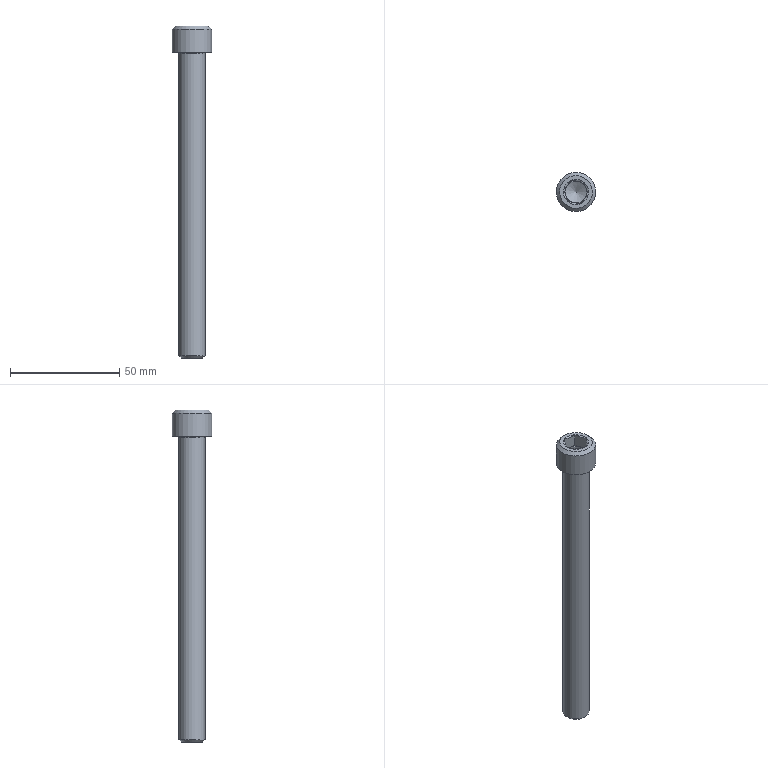Part | NX | features solid 2 | 1 solid | 32 faces | box 18 x 18 x 152 mm | volume 18123 mm3 | plane 19 | cone 9 | cylinder 3 | torus 1 | commonest cylinder face diameters 10 x1 12 x1 18 x1
STEP:
#1=CARTESIAN_POINT('',(532.671,620.304,196.));
#2=VERTEX_POINT('',#1);
#3=CARTESIAN_POINT('',(531.842,622.582,196.));
#4=VERTEX_POINT('',#3);
#5=CARTESIAN_POINT('',(533.817,617.157,196.));
#6=DIRECTION('',(-0.342,0.9397,0.));
#7=VECTOR('',#6,1000.);
#8=LINE('',#5,#7);
#9=EDGE_CURVE('',#2,#4,#8,.T.);
#10=ORIENTED_EDGE('',*,*,#9,.T.);
#11=CARTESIAN_POINT('',(529.455,623.003,196.));
#12=VERTEX_POINT('',#11);
#13=CARTESIAN_POINT('',(526.156,623.585,196.));
#14=DIRECTION('',(0.9848,-0.1736,0.));
#15=VECTOR('',#14,1000.);
#16=LINE('',#13,#15);
#17=EDGE_CURVE('',#12,#4,#16,.T.);
#18=ORIENTED_EDGE('',*,*,#17,.F.);
#19=CARTESIAN_POINT('',(528.146,618.178,196.));
#20=DIRECTION('',(0.,0.,1.));
#21=DIRECTION('',(0.766,-0.6428,0.));
#22=AXIS2_PLACEMENT_3D('',#19,#20,#21);
#23=CIRCLE('',#22,5.);
#24=EDGE_CURVE('',#2,#12,#23,.T.);
#25=ORIENTED_EDGE('',*,*,#24,.F.);
#26=EDGE_LOOP('',(#10,#18,#25));
#27=FACE_BOUND('',#26,.T.);
#28=CARTESIAN_POINT('',(528.146,618.178,196.));
#29=DIRECTION('',(0.,0.,1.));
#30=DIRECTION('',(-0.766,0.6428,0.));
#31=AXIS2_PLACEMENT_3D('',#28,#29,#30);
#32=PLANE('',#31);
#33=ADVANCED_FACE('',(#27),#32,.T.);
#34=CARTESIAN_POINT('',(526.156,623.585,196.));
#35=VERTEX_POINT('',#34);
#36=CARTESIAN_POINT('',(528.567,623.16,196.));
#37=VERTEX_POINT('',#36);
#38=CARTESIAN_POINT('',(526.156,623.585,196.));
#39=DIRECTION('',(0.9848,-0.1736,0.));
#40=VECTOR('',#39,1000.);
#41=LINE('',#38,#40);
#42=EDGE_CURVE('',#35,#37,#41,.T.);
#43=ORIENTED_EDGE('',*,*,#42,.F.);
#44=CARTESIAN_POINT('',(524.316,621.391,196.));
#45=VERTEX_POINT('',#44);
#46=CARTESIAN_POINT('',(522.475,619.198,196.));
#47=DIRECTION('',(0.6428,0.766,0.));
#48=VECTOR('',#47,1000.);
#49=LINE('',#46,#48);
#50=EDGE_CURVE('',#45,#35,#49,.T.);
#51=ORIENTED_EDGE('',*,*,#50,.F.);
#52=CARTESIAN_POINT('',(528.146,618.178,196.));
#53=DIRECTION('',(0.,0.,1.));
#54=DIRECTION('',(0.766,-0.6428,0.));
#55=AXIS2_PLACEMENT_3D('',#52,#53,#54);
#56=CIRCLE('',#55,5.);
#57=EDGE_CURVE('',#37,#45,#56,.T.);
#58=ORIENTED_EDGE('',*,*,#57,.F.);
#59=EDGE_LOOP('',(#43,#51,#58));
#60=FACE_BOUND('',#59,.T.);
#61=CARTESIAN_POINT('',(528.146,618.178,196.));
#62=DIRECTION('',(0.,0.,1.));
#63=DIRECTION('',(-0.766,0.6428,0.));
#64=AXIS2_PLACEMENT_3D('',#61,#62,#63);
#65=PLANE('',#64);
#66=ADVANCED_FACE('',(#60),#65,.T.);
#67=CARTESIAN_POINT('',(522.475,619.198,196.));
#68=VERTEX_POINT('',#67);
#69=CARTESIAN_POINT('',(522.475,619.198,196.));
#70=DIRECTION('',(0.6428,0.766,0.));
#71=VECTOR('',#70,1000.);
#72=LINE('',#69,#71);
#73=EDGE_CURVE('',#68,#45,#72,.T.);
#74=ORIENTED_EDGE('',*,*,#73,.F.);
#75=CARTESIAN_POINT('',(523.312,616.898,196.));
#76=VERTEX_POINT('',#75);
#77=CARTESIAN_POINT('',(524.45,613.773,196.));
#78=DIRECTION('',(-0.342,0.9397,0.));
#79=VECTOR('',#78,1000.);
#80=LINE('',#77,#79);
#81=EDGE_CURVE('',#76,#68,#80,.T.);
#82=ORIENTED_EDGE('',*,*,#81,.F.);
#83=CARTESIAN_POINT('',(528.146,618.178,196.));
#84=DIRECTION('',(0.,0.,1.));
#85=DIRECTION('',(0.766,-0.6428,0.));
#86=AXIS2_PLACEMENT_3D('',#83,#84,#85);
#87=CIRCLE('',#86,5.);
#88=EDGE_CURVE('',#45,#76,#87,.T.);
#89=ORIENTED_EDGE('',*,*,#88,.F.);
#90=EDGE_LOOP('',(#74,#82,#89));
#91=FACE_BOUND('',#90,.T.);
#92=CARTESIAN_POINT('',(528.146,618.178,196.));
#93=DIRECTION('',(0.,0.,1.));
#94=DIRECTION('',(-0.766,0.6428,0.));
#95=AXIS2_PLACEMENT_3D('',#92,#93,#94);
#96=PLANE('',#95);
#97=ADVANCED_FACE('',(#91),#96,.T.);
#98=CARTESIAN_POINT('',(524.45,613.773,196.));
#99=VERTEX_POINT('',#98);
#100=CARTESIAN_POINT('',(523.621,616.051,196.));
#101=VERTEX_POINT('',#100);
#102=CARTESIAN_POINT('',(524.45,613.773,196.));
#103=DIRECTION('',(-0.342,0.9397,0.));
#104=VECTOR('',#103,1000.);
#105=LINE('',#102,#104);
#106=EDGE_CURVE('',#99,#101,#105,.T.);
#107=ORIENTED_EDGE('',*,*,#106,.F.);
#108=CARTESIAN_POINT('',(526.837,613.352,196.));
#109=VERTEX_POINT('',#108);
#110=CARTESIAN_POINT('',(530.136,612.77,196.));
#111=DIRECTION('',(-0.9848,0.1736,0.));
#112=VECTOR('',#111,1000.);
#113=LINE('',#110,#112);
#114=EDGE_CURVE('',#109,#99,#113,.T.);
#115=ORIENTED_EDGE('',*,*,#114,.F.);
#116=CARTESIAN_POINT('',(528.146,618.178,196.));
#117=DIRECTION('',(0.,0.,1.));
#118=DIRECTION('',(0.766,-0.6428,0.));
#119=AXIS2_PLACEMENT_3D('',#116,#117,#118);
#120=CIRCLE('',#119,5.);
#121=EDGE_CURVE('',#101,#109,#120,.T.);
#122=ORIENTED_EDGE('',*,*,#121,.F.);
#123=EDGE_LOOP('',(#107,#115,#122));
#124=FACE_BOUND('',#123,.T.);
#125=CARTESIAN_POINT('',(528.146,618.178,196.));
#126=DIRECTION('',(0.,0.,1.));
#127=DIRECTION('',(-0.766,0.6428,0.));
#128=AXIS2_PLACEMENT_3D('',#125,#126,#127);
#129=PLANE('',#128);
#130=ADVANCED_FACE('',(#124),#129,.T.);
#131=CARTESIAN_POINT('',(533.817,617.157,196.));
#132=VERTEX_POINT('',#131);
#133=CARTESIAN_POINT('',(531.976,614.964,196.));
#134=VERTEX_POINT('',#133);
#135=CARTESIAN_POINT('',(533.817,617.157,196.));
#136=DIRECTION('',(-0.6428,-0.766,0.));
#137=VECTOR('',#136,1000.);
#138=LINE('',#135,#137);
#139=EDGE_CURVE('',#132,#134,#138,.T.);
#140=ORIENTED_EDGE('',*,*,#139,.F.);
#141=CARTESIAN_POINT('',(532.979,619.457,196.));
#142=VERTEX_POINT('',#141);
#143=CARTESIAN_POINT('',(533.817,617.157,196.));
#144=DIRECTION('',(-0.342,0.9397,0.));
#145=VECTOR('',#144,1000.);
#146=LINE('',#143,#145);
#147=EDGE_CURVE('',#132,#142,#146,.T.);
#148=ORIENTED_EDGE('',*,*,#147,.T.);
#149=CARTESIAN_POINT('',(528.146,618.178,196.));
#150=DIRECTION('',(0.,0.,1.));
#151=DIRECTION('',(0.766,-0.6428,0.));
#152=AXIS2_PLACEMENT_3D('',#149,#150,#151);
#153=CIRCLE('',#152,5.);
#154=EDGE_CURVE('',#134,#142,#153,.T.);
#155=ORIENTED_EDGE('',*,*,#154,.F.);
#156=EDGE_LOOP('',(#140,#148,#155));
#157=FACE_BOUND('',#156,.T.);
#158=CARTESIAN_POINT('',(528.146,618.178,196.));
#159=DIRECTION('',(0.,0.,1.));
#160=DIRECTION('',(-0.766,0.6428,0.));
#161=AXIS2_PLACEMENT_3D('',#158,#159,#160);
#162=PLANE('',#161);
#163=ADVANCED_FACE('',(#157),#162,.T.);
#164=CARTESIAN_POINT('',(530.136,612.77,196.));
#165=VERTEX_POINT('',#164);
#166=CARTESIAN_POINT('',(527.725,613.195,196.));
#167=VERTEX_POINT('',#166);
#168=CARTESIAN_POINT('',(530.136,612.77,196.));
#169=DIRECTION('',(-0.9848,0.1736,0.));
#170=VECTOR('',#169,1000.);
#171=LINE('',#168,#170);
#172=EDGE_CURVE('',#165,#167,#171,.T.);
#173=ORIENTED_EDGE('',*,*,#172,.F.);
#174=CARTESIAN_POINT('',(533.817,617.157,196.));
#175=DIRECTION('',(-0.6428,-0.766,0.));
#176=VECTOR('',#175,1000.);
#177=LINE('',#174,#176);
#178=EDGE_CURVE('',#134,#165,#177,.T.);
#179=ORIENTED_EDGE('',*,*,#178,.F.);
#180=CARTESIAN_POINT('',(528.146,618.178,196.));
#181=DIRECTION('',(0.,0.,1.));
#182=DIRECTION('',(0.766,-0.6428,0.));
#183=AXIS2_PLACEMENT_3D('',#180,#181,#182);
#184=CIRCLE('',#183,5.);
#185=EDGE_CURVE('',#167,#134,#184,.T.);
#186=ORIENTED_EDGE('',*,*,#185,.F.);
#187=EDGE_LOOP('',(#173,#179,#186));
#188=FACE_BOUND('',#187,.T.);
#189=CARTESIAN_POINT('',(528.146,618.178,196.));
#190=DIRECTION('',(0.,0.,1.));
#191=DIRECTION('',(-0.766,0.6428,0.));
#192=AXIS2_PLACEMENT_3D('',#189,#190,#191);
#193=PLANE('',#192);
#194=ADVANCED_FACE('',(#188),#193,.T.);
#195=CARTESIAN_POINT('',(522.475,619.198,202.));
#196=VERTEX_POINT('',#195);
#197=CARTESIAN_POINT('',(522.491,619.216,202.));
#198=VERTEX_POINT('',#197);
#199=CARTESIAN_POINT('',(522.475,619.198,202.));
#200=DIRECTION('',(0.6428,0.766,0.));
#201=VECTOR('',#200,1000.);
#202=LINE('',#199,#201);
#203=EDGE_CURVE('',#196,#198,#202,.T.);
#204=ORIENTED_EDGE('',*,*,#203,.F.);
#205=CARTESIAN_POINT('',(522.475,619.198,196.));
#206=DIRECTION('',(0.,0.,1.));
#207=VECTOR('',#206,1000.);
#208=LINE('',#205,#207);
#209=EDGE_CURVE('',#68,#196,#208,.T.);
#210=ORIENTED_EDGE('',*,*,#209,.F.);
#211=ORIENTED_EDGE('',*,*,#73,.T.);
#212=ORIENTED_EDGE('',*,*,#50,.T.);
#213=CARTESIAN_POINT('',(526.156,623.585,202.));
#214=VERTEX_POINT('',#213);
#215=CARTESIAN_POINT('',(526.156,623.585,196.));
#216=DIRECTION('',(0.,0.,1.));
#217=VECTOR('',#216,1000.);
#218=LINE('',#215,#217);
#219=EDGE_CURVE('',#35,#214,#218,.T.);
#220=ORIENTED_EDGE('',*,*,#219,.T.);
#221=CARTESIAN_POINT('',(526.141,623.567,202.));
#222=VERTEX_POINT('',#221);
#223=CARTESIAN_POINT('',(522.475,619.198,202.));
#224=DIRECTION('',(0.6428,0.766,0.));
#225=VECTOR('',#224,1000.);
#226=LINE('',#223,#225);
#227=EDGE_CURVE('',#222,#214,#226,.T.);
#228=ORIENTED_EDGE('',*,*,#227,.F.);
#229=CARTESIAN_POINT('',(522.491,619.216,202.));
#230=CARTESIAN_POINT('',(523.084,619.924,201.737));
#231=CARTESIAN_POINT('',(524.315,621.39,201.397));
#232=CARTESIAN_POINT('',(525.551,622.863,201.738));
#233=CARTESIAN_POINT('',(526.141,623.567,202.));
#234=B_SPLINE_CURVE_WITH_KNOTS('',3,(#229,#230,#231,#232,#233),.UNSPECIFIED.,.F.,.F.,(4,1,4),(0.004945,0.007815,0.01069),.UNSPECIFIED.);
#235=EDGE_CURVE('',#198,#222,#234,.T.);
#236=ORIENTED_EDGE('',*,*,#235,.F.);
#237=EDGE_LOOP('',(#204,#210,#211,#212,#220,#228,#236));
#238=FACE_BOUND('',#237,.T.);
#239=CARTESIAN_POINT('',(522.475,619.198,196.));
#240=DIRECTION('',(-0.766,0.6428,0.));
#241=DIRECTION('',(0.,0.,-1.));
#242=AXIS2_PLACEMENT_3D('',#239,#240,#241);
#243=PLANE('',#242);
#244=ADVANCED_FACE('',(#238),#243,.F.);
#245=CARTESIAN_POINT('',(524.45,613.773,202.));
#246=VERTEX_POINT('',#245);
#247=CARTESIAN_POINT('',(524.45,613.773,196.));
#248=DIRECTION('',(0.,0.,1.));
#249=VECTOR('',#248,1000.);
#250=LINE('',#247,#249);
#251=EDGE_CURVE('',#99,#246,#250,.T.);
#252=ORIENTED_EDGE('',*,*,#251,.F.);
#253=ORIENTED_EDGE('',*,*,#106,.T.);
#254=CARTESIAN_POINT('',(524.45,613.773,196.));
#255=DIRECTION('',(-0.342,0.9397,0.));
#256=VECTOR('',#255,1000.);
#257=LINE('',#254,#256);
#258=EDGE_CURVE('',#101,#76,#257,.T.);
#259=ORIENTED_EDGE('',*,*,#258,.T.);
#260=ORIENTED_EDGE('',*,*,#81,.T.);
#261=ORIENTED_EDGE('',*,*,#209,.T.);
#262=CARTESIAN_POINT('',(522.483,619.176,202.));
#263=VERTEX_POINT('',#262);
#264=CARTESIAN_POINT('',(524.45,613.773,202.));
#265=DIRECTION('',(-0.342,0.9397,0.));
#266=VECTOR('',#265,1000.);
#267=LINE('',#264,#266);
#268=EDGE_CURVE('',#263,#196,#267,.T.);
#269=ORIENTED_EDGE('',*,*,#268,.F.);
#270=CARTESIAN_POINT('',(524.45,613.773,202.));
#271=CARTESIAN_POINT('',(524.129,614.655,201.729));
#272=CARTESIAN_POINT('',(523.47,616.465,201.382));
#273=CARTESIAN_POINT('',(522.805,618.293,201.729));
#274=CARTESIAN_POINT('',(522.483,619.176,202.));
#275=B_SPLINE_CURVE_WITH_KNOTS('',3,(#270,#271,#272,#273,#274),.UNSPECIFIED.,.F.,.F.,(4,1,4),(0.000000238,0.002904,0.005807),.UNSPECIFIED.);
#276=EDGE_CURVE('',#246,#263,#275,.T.);
#277=ORIENTED_EDGE('',*,*,#276,.F.);
#278=EDGE_LOOP('',(#252,#253,#259,#260,#261,#269,#277));
#279=FACE_BOUND('',#278,.T.);
#280=CARTESIAN_POINT('',(524.45,613.773,196.));
#281=DIRECTION('',(-0.9397,-0.342,0.));
#282=DIRECTION('',(-0.342,0.9397,0.));
#283=AXIS2_PLACEMENT_3D('',#280,#281,#282);
#284=PLANE('',#283);
#285=ADVANCED_FACE('',(#279),#284,.F.);
#286=CARTESIAN_POINT('',(530.136,612.77,202.));
#287=VERTEX_POINT('',#286);
#288=CARTESIAN_POINT('',(530.113,612.774,202.));
#289=VERTEX_POINT('',#288);
#290=CARTESIAN_POINT('',(530.136,612.77,202.));
#291=DIRECTION('',(-0.9848,0.1736,0.));
#292=VECTOR('',#291,1000.);
#293=LINE('',#290,#292);
#294=EDGE_CURVE('',#287,#289,#293,.T.);
#295=ORIENTED_EDGE('',*,*,#294,.F.);
#296=CARTESIAN_POINT('',(530.136,612.77,196.));
#297=DIRECTION('',(0.,0.,1.));
#298=VECTOR('',#297,1000.);
#299=LINE('',#296,#298);
#300=EDGE_CURVE('',#165,#287,#299,.T.);
#301=ORIENTED_EDGE('',*,*,#300,.F.);
#302=ORIENTED_EDGE('',*,*,#172,.T.);
#303=CARTESIAN_POINT('',(530.136,612.77,196.));
#304=DIRECTION('',(-0.9848,0.1736,0.));
#305=VECTOR('',#304,1000.);
#306=LINE('',#303,#305);
#307=EDGE_CURVE('',#167,#109,#306,.T.);
#308=ORIENTED_EDGE('',*,*,#307,.T.);
#309=ORIENTED_EDGE('',*,*,#114,.T.);
#310=ORIENTED_EDGE('',*,*,#251,.T.);
#311=CARTESIAN_POINT('',(530.113,612.774,202.));
#312=CARTESIAN_POINT('',(529.188,612.937,201.729));
#313=CARTESIAN_POINT('',(527.292,613.272,201.382));
#314=CARTESIAN_POINT('',(525.376,613.61,201.729));
#315=CARTESIAN_POINT('',(524.45,613.773,202.));
#316=B_SPLINE_CURVE_WITH_KNOTS('',3,(#311,#312,#313,#314,#315),.UNSPECIFIED.,.F.,.F.,(4,1,4),(0.000000714,0.002904,0.005808),.UNSPECIFIED.);
#317=EDGE_CURVE('',#289,#246,#316,.T.);
#318=ORIENTED_EDGE('',*,*,#317,.F.);
#319=EDGE_LOOP('',(#295,#301,#302,#308,#309,#310,#318));
#320=FACE_BOUND('',#319,.T.);
#321=CARTESIAN_POINT('',(530.136,612.77,196.));
#322=DIRECTION('',(-0.1736,-0.9848,0.));
#323=DIRECTION('',(-0.9848,0.1736,0.));
#324=AXIS2_PLACEMENT_3D('',#321,#322,#323);
#325=PLANE('',#324);
#326=ADVANCED_FACE('',(#320),#325,.F.);
#327=CARTESIAN_POINT('',(533.817,617.157,202.));
#328=VERTEX_POINT('',#327);
#329=CARTESIAN_POINT('',(533.801,617.139,202.));
#330=VERTEX_POINT('',#329);
#331=CARTESIAN_POINT('',(533.817,617.157,202.));
#332=DIRECTION('',(-0.6428,-0.766,0.));
#333=VECTOR('',#332,1000.);
#334=LINE('',#331,#333);
#335=EDGE_CURVE('',#328,#330,#334,.T.);
#336=ORIENTED_EDGE('',*,*,#335,.F.);
#337=CARTESIAN_POINT('',(533.817,617.157,196.));
#338=DIRECTION('',(0.,0.,1.));
#339=VECTOR('',#338,1000.);
#340=LINE('',#337,#339);
#341=EDGE_CURVE('',#132,#328,#340,.T.);
#342=ORIENTED_EDGE('',*,*,#341,.F.);
#343=ORIENTED_EDGE('',*,*,#139,.T.);
#344=ORIENTED_EDGE('',*,*,#178,.T.);
#345=ORIENTED_EDGE('',*,*,#300,.T.);
#346=CARTESIAN_POINT('',(530.151,612.788,202.));
#347=VERTEX_POINT('',#346);
#348=CARTESIAN_POINT('',(533.817,617.157,202.));
#349=DIRECTION('',(-0.6428,-0.766,0.));
#350=VECTOR('',#349,1000.);
#351=LINE('',#348,#350);
#352=EDGE_CURVE('',#347,#287,#351,.T.);
#353=ORIENTED_EDGE('',*,*,#352,.F.);
#354=CARTESIAN_POINT('',(530.151,612.788,202.));
#355=CARTESIAN_POINT('',(530.745,613.496,201.737));
#356=CARTESIAN_POINT('',(531.975,614.963,201.397));
#357=CARTESIAN_POINT('',(533.211,616.435,201.738));
#358=CARTESIAN_POINT('',(533.801,617.139,202.));
#359=B_SPLINE_CURVE_WITH_KNOTS('',3,(#354,#355,#356,#357,#358),.UNSPECIFIED.,.F.,.F.,(4,1,4),(0.004945,0.007815,0.01069),.UNSPECIFIED.);
#360=EDGE_CURVE('',#330,#347,#359,.F.);
#361=ORIENTED_EDGE('',*,*,#360,.F.);
#362=EDGE_LOOP('',(#336,#342,#343,#344,#345,#353,#361));
#363=FACE_BOUND('',#362,.T.);
#364=CARTESIAN_POINT('',(533.817,617.157,196.));
#365=DIRECTION('',(0.766,-0.6428,0.));
#366=DIRECTION('',(0.,0.,1.));
#367=AXIS2_PLACEMENT_3D('',#364,#365,#366);
#368=PLANE('',#367);
#369=ADVANCED_FACE('',(#363),#368,.F.);
#370=CARTESIAN_POINT('',(533.809,617.179,202.));
#371=VERTEX_POINT('',#370);
#372=CARTESIAN_POINT('',(531.842,622.582,202.));
#373=VERTEX_POINT('',#372);
#374=CARTESIAN_POINT('',(533.809,617.179,202.));
#375=CARTESIAN_POINT('',(533.488,618.061,201.729));
#376=CARTESIAN_POINT('',(532.829,619.871,201.382));
#377=CARTESIAN_POINT('',(532.164,621.699,201.729));
#378=CARTESIAN_POINT('',(531.842,622.582,202.));
#379=B_SPLINE_CURVE_WITH_KNOTS('',3,(#374,#375,#376,#377,#378),.UNSPECIFIED.,.F.,.F.,(4,1,4),(0.000000714,0.002904,0.005808),.UNSPECIFIED.);
#380=EDGE_CURVE('',#371,#373,#379,.T.);
#381=ORIENTED_EDGE('',*,*,#380,.T.);
#382=CARTESIAN_POINT('',(531.842,622.582,196.));
#383=DIRECTION('',(0.,0.,1.));
#384=VECTOR('',#383,1000.);
#385=LINE('',#382,#384);
#386=EDGE_CURVE('',#4,#373,#385,.T.);
#387=ORIENTED_EDGE('',*,*,#386,.F.);
#388=ORIENTED_EDGE('',*,*,#9,.F.);
#389=CARTESIAN_POINT('',(533.817,617.157,196.));
#390=DIRECTION('',(-0.342,0.9397,0.));
#391=VECTOR('',#390,1000.);
#392=LINE('',#389,#391);
#393=EDGE_CURVE('',#142,#2,#392,.T.);
#394=ORIENTED_EDGE('',*,*,#393,.F.);
#395=ORIENTED_EDGE('',*,*,#147,.F.);
#396=ORIENTED_EDGE('',*,*,#341,.T.);
#397=CARTESIAN_POINT('',(533.817,617.157,202.));
#398=DIRECTION('',(-0.342,0.9397,0.));
#399=VECTOR('',#398,1000.);
#400=LINE('',#397,#399);
#401=EDGE_CURVE('',#328,#371,#400,.T.);
#402=ORIENTED_EDGE('',*,*,#401,.T.);
#403=EDGE_LOOP('',(#381,#387,#388,#394,#395,#396,#402));
#404=FACE_BOUND('',#403,.T.);
#405=CARTESIAN_POINT('',(533.817,617.157,196.));
#406=DIRECTION('',(-0.9397,-0.342,0.));
#407=DIRECTION('',(-0.342,0.9397,0.));
#408=AXIS2_PLACEMENT_3D('',#405,#406,#407);
#409=PLANE('',#408);
#410=ADVANCED_FACE('',(#404),#409,.T.);
#411=CARTESIAN_POINT('',(526.179,623.581,202.));
#412=VERTEX_POINT('',#411);
#413=CARTESIAN_POINT('',(526.156,623.585,202.));
#414=DIRECTION('',(0.9848,-0.1736,0.));
#415=VECTOR('',#414,1000.);
#416=LINE('',#413,#415);
#417=EDGE_CURVE('',#214,#412,#416,.T.);
#418=ORIENTED_EDGE('',*,*,#417,.F.);
#419=ORIENTED_EDGE('',*,*,#219,.F.);
#420=ORIENTED_EDGE('',*,*,#42,.T.);
#421=CARTESIAN_POINT('',(526.156,623.585,196.));
#422=DIRECTION('',(0.9848,-0.1736,0.));
#423=VECTOR('',#422,1000.);
#424=LINE('',#421,#423);
#425=EDGE_CURVE('',#37,#12,#424,.T.);
#426=ORIENTED_EDGE('',*,*,#425,.T.);
#427=ORIENTED_EDGE('',*,*,#17,.T.);
#428=ORIENTED_EDGE('',*,*,#386,.T.);
#429=CARTESIAN_POINT('',(526.179,623.581,202.));
#430=CARTESIAN_POINT('',(527.104,623.418,201.729));
#431=CARTESIAN_POINT('',(529.,623.083,201.382));
#432=CARTESIAN_POINT('',(530.916,622.746,201.729));
#433=CARTESIAN_POINT('',(531.842,622.582,202.));
#434=B_SPLINE_CURVE_WITH_KNOTS('',3,(#429,#430,#431,#432,#433),.UNSPECIFIED.,.F.,.F.,(4,1,4),(0.000000714,0.002904,0.005808),.UNSPECIFIED.);
#435=EDGE_CURVE('',#412,#373,#434,.T.);
#436=ORIENTED_EDGE('',*,*,#435,.F.);
#437=EDGE_LOOP('',(#418,#419,#420,#426,#427,#428,#436));
#438=FACE_BOUND('',#437,.T.);
#439=CARTESIAN_POINT('',(526.156,623.585,196.));
#440=DIRECTION('',(0.1736,0.9848,0.));
#441=DIRECTION('',(0.9848,-0.1736,0.));
#442=AXIS2_PLACEMENT_3D('',#439,#440,#441);
#443=PLANE('',#442);
#444=ADVANCED_FACE('',(#438),#443,.F.);
#445=CARTESIAN_POINT('',(521.252,623.963,200.5));
#446=VERTEX_POINT('',#445);
#447=CARTESIAN_POINT('',(528.146,618.178,200.5));
#448=DIRECTION('',(0.,0.,-1.));
#449=DIRECTION('',(-0.766,0.6428,0.));
#450=AXIS2_PLACEMENT_3D('',#447,#448,#449);
#451=CIRCLE('',#450,9.);
#452=EDGE_CURVE('',#446,#446,#451,.F.);
#453=ORIENTED_EDGE('',*,*,#452,.F.);
#454=EDGE_LOOP('',(#453));
#455=FACE_BOUND('',#454,.T.);
#456=CARTESIAN_POINT('',(535.04,612.392,190.));
#457=VERTEX_POINT('',#456);
#458=CARTESIAN_POINT('',(528.146,618.178,190.));
#459=DIRECTION('',(0.,0.,1.));
#460=DIRECTION('',(0.766,-0.6428,0.));
#461=AXIS2_PLACEMENT_3D('',#458,#459,#460);
#462=CIRCLE('',#461,9.);
#463=EDGE_CURVE('',#457,#457,#462,.T.);
#464=ORIENTED_EDGE('',*,*,#463,.T.);
#465=EDGE_LOOP('',(#464));
#466=FACE_BOUND('',#465,.T.);
#467=CARTESIAN_POINT('',(528.146,618.178,196.));
#468=DIRECTION('',(0.,0.,1.));
#469=DIRECTION('',(-0.766,0.6428,0.));
#470=AXIS2_PLACEMENT_3D('',#467,#468,#469);
#471=CYLINDRICAL_SURFACE('',#470,9.);
#472=ADVANCED_FACE('',(#455,#466),#471,.T.);
#473=CARTESIAN_POINT('',(528.146,618.178,202.));
#474=DIRECTION('',(0.,0.,-1.));
#475=DIRECTION('',(-0.766,0.6428,0.));
#476=AXIS2_PLACEMENT_3D('',#473,#474,#475);
#477=CIRCLE('',#476,5.75);
#478=EDGE_CURVE('',#412,#373,#477,.T.);
#479=ORIENTED_EDGE('',*,*,#478,.T.);
#480=CARTESIAN_POINT('',(528.146,618.178,202.));
#481=DIRECTION('',(0.,0.,1.));
#482=DIRECTION('',(0.766,-0.6428,0.));
#483=AXIS2_PLACEMENT_3D('',#480,#481,#482);
#484=CIRCLE('',#483,5.75);
#485=EDGE_CURVE('',#371,#373,#484,.T.);
#486=ORIENTED_EDGE('',*,*,#485,.F.);
#487=ORIENTED_EDGE('',*,*,#401,.F.);
#488=ORIENTED_EDGE('',*,*,#335,.T.);
#489=CARTESIAN_POINT('',(528.146,618.178,202.));
#490=DIRECTION('',(0.,0.,-1.));
#491=DIRECTION('',(-0.766,0.6428,0.));
#492=AXIS2_PLACEMENT_3D('',#489,#490,#491);
#493=CIRCLE('',#492,5.75);
#494=EDGE_CURVE('',#330,#347,#493,.T.);
#495=ORIENTED_EDGE('',*,*,#494,.T.);
#496=ORIENTED_EDGE('',*,*,#352,.T.);
#497=ORIENTED_EDGE('',*,*,#294,.T.);
#498=CARTESIAN_POINT('',(528.146,618.178,202.));
#499=DIRECTION('',(0.,0.,-1.));
#500=DIRECTION('',(-0.766,0.6428,0.));
#501=AXIS2_PLACEMENT_3D('',#498,#499,#500);
#502=CIRCLE('',#501,5.75);
#503=EDGE_CURVE('',#289,#246,#502,.T.);
#504=ORIENTED_EDGE('',*,*,#503,.T.);
#505=CARTESIAN_POINT('',(528.146,618.178,202.));
#506=DIRECTION('',(0.,0.,-1.));
#507=DIRECTION('',(-0.766,0.6428,0.));
#508=AXIS2_PLACEMENT_3D('',#505,#506,#507);
#509=CIRCLE('',#508,5.75);
#510=EDGE_CURVE('',#246,#263,#509,.T.);
#511=ORIENTED_EDGE('',*,*,#510,.T.);
#512=ORIENTED_EDGE('',*,*,#268,.T.);
#513=ORIENTED_EDGE('',*,*,#203,.T.);
#514=CARTESIAN_POINT('',(528.146,618.178,202.));
#515=DIRECTION('',(0.,0.,-1.));
#516=DIRECTION('',(-0.766,0.6428,0.));
#517=AXIS2_PLACEMENT_3D('',#514,#515,#516);
#518=CIRCLE('',#517,5.75);
#519=EDGE_CURVE('',#198,#222,#518,.T.);
#520=ORIENTED_EDGE('',*,*,#519,.T.);
#521=ORIENTED_EDGE('',*,*,#227,.T.);
#522=ORIENTED_EDGE('',*,*,#417,.T.);
#523=EDGE_LOOP('',(#479,#486,#487,#488,#495,#496,#497,#504,#511,#512,#513,#520,#521,#522));
#524=FACE_BOUND('',#523,.T.);
#525=CARTESIAN_POINT('',(522.401,622.998,202.));
#526=VERTEX_POINT('',#525);
#527=CARTESIAN_POINT('',(528.146,618.178,202.));
#528=DIRECTION('',(0.,0.,-1.));
#529=DIRECTION('',(-0.766,0.6428,0.));
#530=AXIS2_PLACEMENT_3D('',#527,#528,#529);
#531=CIRCLE('',#530,7.5);
#532=EDGE_CURVE('',#526,#526,#531,.T.);
#533=ORIENTED_EDGE('',*,*,#532,.F.);
#534=EDGE_LOOP('',(#533));
#535=FACE_BOUND('',#534,.T.);
#536=CARTESIAN_POINT('',(528.146,618.178,202.));
#537=DIRECTION('',(0.,0.,1.));
#538=DIRECTION('',(-0.766,0.6428,0.));
#539=AXIS2_PLACEMENT_3D('',#536,#537,#538);
#540=PLANE('',#539);
#541=ADVANCED_FACE('',(#524,#535),#540,.T.);
#542=CARTESIAN_POINT('',(533.202,613.935,190.));
#543=VERTEX_POINT('',#542);
#544=CARTESIAN_POINT('',(528.146,618.178,190.));
#545=DIRECTION('',(0.,0.,1.));
#546=DIRECTION('',(0.766,-0.6428,0.));
#547=AXIS2_PLACEMENT_3D('',#544,#545,#546);
#548=CIRCLE('',#547,6.6);
#549=EDGE_CURVE('',#543,#543,#548,.F.);
#550=ORIENTED_EDGE('',*,*,#549,.F.);
#551=EDGE_LOOP('',(#550));
#552=FACE_BOUND('',#551,.T.);
#553=ORIENTED_EDGE('',*,*,#463,.F.);
#554=EDGE_LOOP('',(#553));
#555=FACE_BOUND('',#554,.T.);
#556=CARTESIAN_POINT('',(528.146,618.178,190.));
#557=DIRECTION('',(0.,0.,-1.));
#558=DIRECTION('',(0.766,-0.6428,0.));
#559=AXIS2_PLACEMENT_3D('',#556,#557,#558);
#560=PLANE('',#559);
#561=ADVANCED_FACE('',(#552,#555),#560,.T.);
#562=CARTESIAN_POINT('',(528.146,618.178,196.));
#563=DIRECTION('',(0.,0.,1.));
#564=DIRECTION('',(0.766,-0.6428,0.));
#565=AXIS2_PLACEMENT_3D('',#562,#563,#564);
#566=CIRCLE('',#565,5.);
#567=EDGE_CURVE('',#142,#2,#566,.T.);
#568=ORIENTED_EDGE('',*,*,#567,.F.);
#569=ORIENTED_EDGE('',*,*,#393,.T.);
#570=EDGE_LOOP('',(#568,#569));
#571=FACE_BOUND('',#570,.T.);
#572=CARTESIAN_POINT('',(528.146,618.178,196.));
#573=DIRECTION('',(0.,0.,1.));
#574=DIRECTION('',(-0.766,0.6428,0.));
#575=AXIS2_PLACEMENT_3D('',#572,#573,#574);
#576=PLANE('',#575);
#577=ADVANCED_FACE('',(#571),#576,.F.);
#578=ORIENTED_EDGE('',*,*,#425,.F.);
#579=CARTESIAN_POINT('',(528.146,618.178,196.));
#580=DIRECTION('',(0.,0.,1.));
#581=DIRECTION('',(0.766,-0.6428,0.));
#582=AXIS2_PLACEMENT_3D('',#579,#580,#581);
#583=CIRCLE('',#582,5.);
#584=EDGE_CURVE('',#12,#37,#583,.T.);
#585=ORIENTED_EDGE('',*,*,#584,.F.);
#586=EDGE_LOOP('',(#578,#585));
#587=FACE_BOUND('',#586,.T.);
#588=CARTESIAN_POINT('',(528.146,618.178,196.));
#589=DIRECTION('',(0.,0.,1.));
#590=DIRECTION('',(-0.766,0.6428,0.));
#591=AXIS2_PLACEMENT_3D('',#588,#589,#590);
#592=PLANE('',#591);
#593=ADVANCED_FACE('',(#587),#592,.F.);
#594=ORIENTED_EDGE('',*,*,#307,.F.);
#595=CARTESIAN_POINT('',(528.146,618.178,196.));
#596=DIRECTION('',(0.,0.,1.));
#597=DIRECTION('',(0.766,-0.6428,0.));
#598=AXIS2_PLACEMENT_3D('',#595,#596,#597);
#599=CIRCLE('',#598,5.);
#600=EDGE_CURVE('',#109,#167,#599,.T.);
#601=ORIENTED_EDGE('',*,*,#600,.F.);
#602=EDGE_LOOP('',(#594,#601));
#603=FACE_BOUND('',#602,.T.);
#604=CARTESIAN_POINT('',(528.146,618.178,196.));
#605=DIRECTION('',(0.,0.,1.));
#606=DIRECTION('',(-0.766,0.6428,0.));
#607=AXIS2_PLACEMENT_3D('',#604,#605,#606);
#608=PLANE('',#607);
#609=ADVANCED_FACE('',(#603),#608,.F.);
#610=CARTESIAN_POINT('',(531.976,614.964,194.8));
#611=VERTEX_POINT('',#610);
#612=CARTESIAN_POINT('',(528.146,618.178,194.8));
#613=DIRECTION('',(0.,0.,1.));
#614=DIRECTION('',(0.766,-0.6428,0.));
#615=AXIS2_PLACEMENT_3D('',#612,#613,#614);
#616=CIRCLE('',#615,5.);
#617=EDGE_CURVE('',#611,#611,#616,.T.);
#618=ORIENTED_EDGE('',*,*,#617,.T.);
#619=EDGE_LOOP('',(#618));
#620=FACE_BOUND('',#619,.T.);
#621=CARTESIAN_POINT('',(528.146,618.178,191.913));
#622=VERTEX_POINT('',#621);
#623=VERTEX_LOOP('',#622);
#624=FACE_BOUND('',#623,.T.);
#625=CARTESIAN_POINT('',(528.146,618.178,194.8));
#626=DIRECTION('',(0.,0.,1.));
#627=DIRECTION('',(-0.766,0.6428,0.));
#628=AXIS2_PLACEMENT_3D('',#625,#626,#627);
#629=CONICAL_SURFACE('',#628,5.,1.047);
#630=ADVANCED_FACE('',(#620,#624),#629,.F.);
#631=ORIENTED_EDGE('',*,*,#258,.F.);
#632=CARTESIAN_POINT('',(528.146,618.178,196.));
#633=DIRECTION('',(0.,0.,1.));
#634=DIRECTION('',(0.766,-0.6428,0.));
#635=AXIS2_PLACEMENT_3D('',#632,#633,#634);
#636=CIRCLE('',#635,5.);
#637=EDGE_CURVE('',#76,#101,#636,.T.);
#638=ORIENTED_EDGE('',*,*,#637,.F.);
#639=EDGE_LOOP('',(#631,#638));
#640=FACE_BOUND('',#639,.T.);
#641=CARTESIAN_POINT('',(528.146,618.178,196.));
#642=DIRECTION('',(0.,0.,1.));
#643=DIRECTION('',(-0.766,0.6428,0.));
#644=AXIS2_PLACEMENT_3D('',#641,#642,#643);
#645=PLANE('',#644);
#646=ADVANCED_FACE('',(#640),#645,.F.);
#647=ORIENTED_EDGE('',*,*,#617,.F.);
#648=EDGE_LOOP('',(#647));
#649=FACE_BOUND('',#648,.T.);
#650=ORIENTED_EDGE('',*,*,#154,.T.);
#651=ORIENTED_EDGE('',*,*,#567,.T.);
#652=ORIENTED_EDGE('',*,*,#24,.T.);
#653=ORIENTED_EDGE('',*,*,#584,.T.);
#654=ORIENTED_EDGE('',*,*,#57,.T.);
#655=ORIENTED_EDGE('',*,*,#88,.T.);
#656=ORIENTED_EDGE('',*,*,#637,.T.);
#657=ORIENTED_EDGE('',*,*,#121,.T.);
#658=ORIENTED_EDGE('',*,*,#600,.T.);
#659=ORIENTED_EDGE('',*,*,#185,.T.);
#660=EDGE_LOOP('',(#650,#651,#652,#653,#654,#655,#656,#657,#658,#659));
#661=FACE_BOUND('',#660,.T.);
#662=CARTESIAN_POINT('',(528.146,618.178,196.));
#663=DIRECTION('',(0.,0.,-1.));
#664=DIRECTION('',(0.766,-0.6428,0.));
#665=AXIS2_PLACEMENT_3D('',#662,#663,#664);
#666=CYLINDRICAL_SURFACE('',#665,5.);
#667=ADVANCED_FACE('',(#649,#661),#666,.F.);
#668=CARTESIAN_POINT('',(531.976,614.964,50.));
#669=VERTEX_POINT('',#668);
#670=CARTESIAN_POINT('',(528.146,618.178,50.));
#671=DIRECTION('',(0.,0.,1.));
#672=DIRECTION('',(0.766,-0.6428,0.));
#673=AXIS2_PLACEMENT_3D('',#670,#671,#672);
#674=CIRCLE('',#673,5.);
#675=EDGE_CURVE('',#669,#669,#674,.T.);
#676=ORIENTED_EDGE('',*,*,#675,.F.);
#677=EDGE_LOOP('',(#676));
#678=FACE_BOUND('',#677,.T.);
#679=CARTESIAN_POINT('',(528.146,618.178,50.));
#680=DIRECTION('',(0.,0.,-1.));
#681=DIRECTION('',(0.766,-0.6428,0.));
#682=AXIS2_PLACEMENT_3D('',#679,#680,#681);
#683=PLANE('',#682);
#684=ADVANCED_FACE('',(#678),#683,.T.);
#685=CARTESIAN_POINT('',(532.742,614.321,189.4));
#686=VERTEX_POINT('',#685);
#687=CARTESIAN_POINT('',(528.146,618.178,189.4));
#688=DIRECTION('',(0.,0.,1.));
#689=DIRECTION('',(0.766,-0.6428,0.));
#690=AXIS2_PLACEMENT_3D('',#687,#688,#689);
#691=CIRCLE('',#690,6.);
#692=EDGE_CURVE('',#686,#686,#691,.T.);
#693=ORIENTED_EDGE('',*,*,#692,.F.);
#694=EDGE_LOOP('',(#693));
#695=FACE_BOUND('',#694,.T.);
#696=CARTESIAN_POINT('',(532.742,614.321,51.));
#697=VERTEX_POINT('',#696);
#698=CARTESIAN_POINT('',(528.146,618.178,51.));
#699=DIRECTION('',(0.,0.,1.));
#700=DIRECTION('',(0.766,-0.6428,0.));
#701=AXIS2_PLACEMENT_3D('',#698,#699,#700);
#702=CIRCLE('',#701,6.);
#703=EDGE_CURVE('',#697,#697,#702,.F.);
#704=ORIENTED_EDGE('',*,*,#703,.F.);
#705=EDGE_LOOP('',(#704));
#706=FACE_BOUND('',#705,.T.);
#707=CARTESIAN_POINT('',(528.146,618.178,190.));
#708=DIRECTION('',(0.,0.,-1.));
#709=DIRECTION('',(0.766,-0.6428,0.));
#710=AXIS2_PLACEMENT_3D('',#707,#708,#709);
#711=CYLINDRICAL_SURFACE('',#710,6.);
#712=ADVANCED_FACE('',(#695,#706),#711,.T.);
#713=ORIENTED_EDGE('',*,*,#703,.T.);
#714=EDGE_LOOP('',(#713));
#715=FACE_BOUND('',#714,.T.);
#716=ORIENTED_EDGE('',*,*,#675,.T.);
#717=EDGE_LOOP('',(#716));
#718=FACE_BOUND('',#717,.T.);
#719=CARTESIAN_POINT('',(528.146,618.178,50.));
#720=DIRECTION('',(0.,0.,1.));
#721=DIRECTION('',(-0.766,0.6428,0.));
#722=AXIS2_PLACEMENT_3D('',#719,#720,#721);
#723=CONICAL_SURFACE('',#722,5.,0.7854);
#724=ADVANCED_FACE('',(#715,#718),#723,.T.);
#725=ORIENTED_EDGE('',*,*,#452,.T.);
#726=EDGE_LOOP('',(#725));
#727=FACE_BOUND('',#726,.T.);
#728=ORIENTED_EDGE('',*,*,#532,.T.);
#729=EDGE_LOOP('',(#728));
#730=FACE_BOUND('',#729,.T.);
#731=CARTESIAN_POINT('',(528.146,618.178,202.));
#732=DIRECTION('',(0.,0.,-1.));
#733=DIRECTION('',(0.766,-0.6428,0.));
#734=AXIS2_PLACEMENT_3D('',#731,#732,#733);
#735=CONICAL_SURFACE('',#734,7.5,0.7854);
#736=ADVANCED_FACE('',(#727,#730),#735,.T.);
#737=ORIENTED_EDGE('',*,*,#549,.T.);
#738=EDGE_LOOP('',(#737));
#739=FACE_BOUND('',#738,.T.);
#740=ORIENTED_EDGE('',*,*,#692,.T.);
#741=EDGE_LOOP('',(#740));
#742=FACE_BOUND('',#741,.T.);
#743=CARTESIAN_POINT('',(528.146,618.178,189.4));
#744=DIRECTION('',(0.,0.,-1.));
#745=DIRECTION('',(0.766,-0.6428,0.));
#746=AXIS2_PLACEMENT_3D('',#743,#744,#745);
#747=TOROIDAL_SURFACE('',#746,6.6,0.6);
#748=ADVANCED_FACE('',(#739,#742),#747,.F.);
#749=ORIENTED_EDGE('',*,*,#519,.F.);
#750=ORIENTED_EDGE('',*,*,#235,.T.);
#751=EDGE_LOOP('',(#749,#750));
#752=FACE_BOUND('',#751,.T.);
#753=CARTESIAN_POINT('',(528.146,618.178,198.68));
#754=DIRECTION('',(0.,0.,1.));
#755=DIRECTION('',(-0.766,0.6428,0.));
#756=AXIS2_PLACEMENT_3D('',#753,#754,#755);
#757=CONICAL_SURFACE('',#756,0.,1.047);
#758=ADVANCED_FACE('',(#752),#757,.F.);
#759=ORIENTED_EDGE('',*,*,#510,.F.);
#760=ORIENTED_EDGE('',*,*,#276,.T.);
#761=EDGE_LOOP('',(#759,#760));
#762=FACE_BOUND('',#761,.T.);
#763=CARTESIAN_POINT('',(528.146,618.178,198.68));
#764=DIRECTION('',(0.,0.,1.));
#765=DIRECTION('',(-0.766,0.6428,0.));
#766=AXIS2_PLACEMENT_3D('',#763,#764,#765);
#767=CONICAL_SURFACE('',#766,0.,1.047);
#768=ADVANCED_FACE('',(#762),#767,.F.);
#769=ORIENTED_EDGE('',*,*,#503,.F.);
#770=ORIENTED_EDGE('',*,*,#317,.T.);
#771=EDGE_LOOP('',(#769,#770));
#772=FACE_BOUND('',#771,.T.);
#773=CARTESIAN_POINT('',(528.146,618.178,198.68));
#774=DIRECTION('',(0.,0.,1.));
#775=DIRECTION('',(-0.766,0.6428,0.));
#776=AXIS2_PLACEMENT_3D('',#773,#774,#775);
#777=CONICAL_SURFACE('',#776,0.,1.047);
#778=ADVANCED_FACE('',(#772),#777,.F.);
#779=ORIENTED_EDGE('',*,*,#494,.F.);
#780=ORIENTED_EDGE('',*,*,#360,.T.);
#781=EDGE_LOOP('',(#779,#780));
#782=FACE_BOUND('',#781,.T.);
#783=CARTESIAN_POINT('',(528.146,618.178,198.68));
#784=DIRECTION('',(0.,0.,1.));
#785=DIRECTION('',(-0.766,0.6428,0.));
#786=AXIS2_PLACEMENT_3D('',#783,#784,#785);
#787=CONICAL_SURFACE('',#786,0.,1.047);
#788=ADVANCED_FACE('',(#782),#787,.F.);
#789=ORIENTED_EDGE('',*,*,#380,.F.);
#790=ORIENTED_EDGE('',*,*,#485,.T.);
#791=EDGE_LOOP('',(#789,#790));
#792=FACE_BOUND('',#791,.T.);
#793=CARTESIAN_POINT('',(528.146,618.178,198.68));
#794=DIRECTION('',(0.,0.,1.));
#795=DIRECTION('',(-0.766,0.6428,0.));
#796=AXIS2_PLACEMENT_3D('',#793,#794,#795);
#797=CONICAL_SURFACE('',#796,0.,1.047);
#798=ADVANCED_FACE('',(#792),#797,.F.);
#799=ORIENTED_EDGE('',*,*,#478,.F.);
#800=ORIENTED_EDGE('',*,*,#435,.T.);
#801=EDGE_LOOP('',(#799,#800));
#802=FACE_BOUND('',#801,.T.);
#803=CARTESIAN_POINT('',(528.146,618.178,198.68));
#804=DIRECTION('',(0.,0.,1.));
#805=DIRECTION('',(-0.766,0.6428,0.));
#806=AXIS2_PLACEMENT_3D('',#803,#804,#805);
#807=CONICAL_SURFACE('',#806,0.,1.047);
#808=ADVANCED_FACE('',(#802),#807,.F.);
#809=CLOSED_SHELL('',(#33,#66,#97,#130,#163,#194,#244,#285,#326,#369,#410,#444,#472,#541,#561,#577,#593,#609,#630,#646,#667,#684,#712,#724,#736,#748,#758,#768,#778,#788,#798,#808));
#810=MANIFOLD_SOLID_BREP('',#809);
#811=(LENGTH_UNIT()NAMED_UNIT(*)SI_UNIT(.MILLI.,.METRE.));
#812=UNCERTAINTY_MEASURE_WITH_UNIT(LENGTH_MEASURE(0.0508),#811,'','');
#813=(NAMED_UNIT(*)PLANE_ANGLE_UNIT()SI_UNIT($,.RADIAN.));
#814=(NAMED_UNIT(*)SI_UNIT($,.STERADIAN.)SOLID_ANGLE_UNIT());
#815=(GEOMETRIC_REPRESENTATION_CONTEXT(3)GLOBAL_UNCERTAINTY_ASSIGNED_CONTEXT((#812))GLOBAL_UNIT_ASSIGNED_CONTEXT((#811,#813,#814))REPRESENTATION_CONTEXT('',''));
#816=ADVANCED_BREP_SHAPE_REPRESENTATION('',(#810),#815);